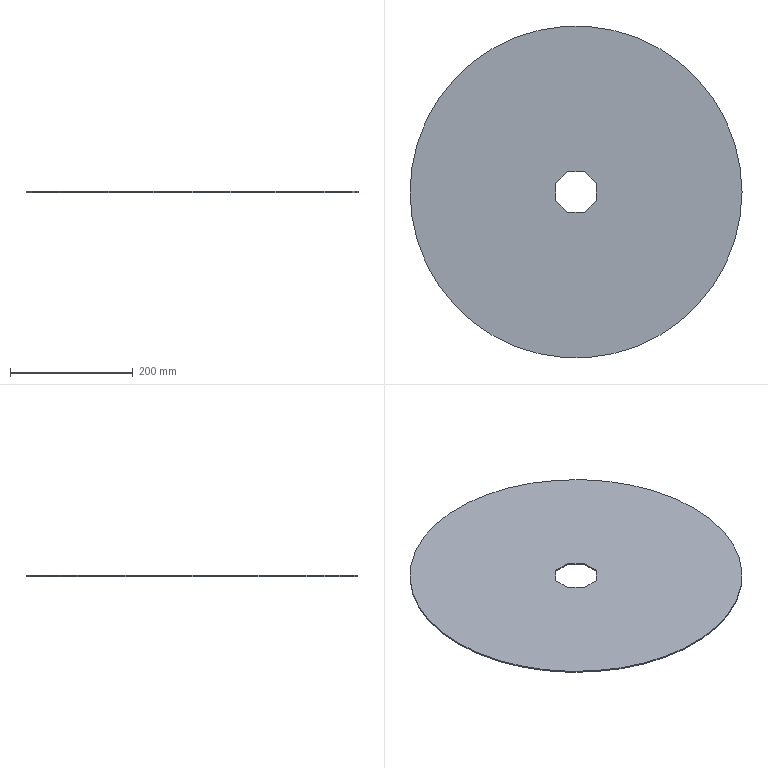Part | SolidWorks | features Extrusion 1 | 1 solid | 12 faces | box 540 x 540 x 2 mm | volume 450713 mm3 | plane 10 | cylinder 2 | commonest cylinder face diameters 540 x2
STEP:
#1=CARTESIAN_POINT('',(270.,0.,2.));
#2=VERTEX_POINT('',#1);
#3=CARTESIAN_POINT('',(-270.,0.,2.));
#4=VERTEX_POINT('',#3);
#5=CARTESIAN_POINT('',(0.,0.,2.));
#6=DIRECTION('',(0.,0.,1.));
#7=DIRECTION('',(1.,0.,0.));
#8=AXIS2_PLACEMENT_3D('',#5,#6,#7);
#9=CIRCLE('',#8,270.);
#10=EDGE_CURVE('',#2,#4,#9,.T.);
#11=ORIENTED_EDGE('',*,*,#10,.F.);
#12=CARTESIAN_POINT('',(270.,0.,0.));
#13=VERTEX_POINT('',#12);
#14=CARTESIAN_POINT('',(270.,0.,2.));
#15=DIRECTION('',(0.,0.,-1.));
#16=VECTOR('',#15,1000.);
#17=LINE('',#14,#16);
#18=EDGE_CURVE('',#2,#13,#17,.T.);
#19=ORIENTED_EDGE('',*,*,#18,.T.);
#20=CARTESIAN_POINT('',(-270.,0.,0.));
#21=VERTEX_POINT('',#20);
#22=CARTESIAN_POINT('',(0.,0.,0.));
#23=DIRECTION('',(0.,0.,1.));
#24=DIRECTION('',(1.,0.,0.));
#25=AXIS2_PLACEMENT_3D('',#22,#23,#24);
#26=CIRCLE('',#25,270.);
#27=EDGE_CURVE('',#13,#21,#26,.T.);
#28=ORIENTED_EDGE('',*,*,#27,.T.);
#29=CARTESIAN_POINT('',(-270.,0.,2.));
#30=DIRECTION('',(0.,0.,-1.));
#31=VECTOR('',#30,1000.);
#32=LINE('',#29,#31);
#33=EDGE_CURVE('',#4,#21,#32,.T.);
#34=ORIENTED_EDGE('',*,*,#33,.F.);
#35=EDGE_LOOP('',(#11,#19,#28,#34));
#36=FACE_OUTER_BOUND('',#35,.T.);
#37=CARTESIAN_POINT('',(0.,0.,2.));
#38=DIRECTION('',(0.,0.,-1.));
#39=DIRECTION('',(-1.,0.,0.));
#40=AXIS2_PLACEMENT_3D('',#37,#38,#39);
#41=CYLINDRICAL_SURFACE('',#40,270.);
#42=ADVANCED_FACE('',(#36),#41,.T.);
#43=CARTESIAN_POINT('',(0.,0.,2.));
#44=DIRECTION('',(0.,0.,1.));
#45=DIRECTION('',(1.,0.,0.));
#46=AXIS2_PLACEMENT_3D('',#43,#44,#45);
#47=CIRCLE('',#46,270.);
#48=EDGE_CURVE('',#4,#2,#47,.T.);
#49=ORIENTED_EDGE('',*,*,#48,.T.);
#50=ORIENTED_EDGE('',*,*,#10,.T.);
#51=EDGE_LOOP('',(#49,#50));
#52=FACE_OUTER_BOUND('',#51,.T.);
#53=CARTESIAN_POINT('',(-13.777,33.26,2.));
#54=VERTEX_POINT('',#53);
#55=CARTESIAN_POINT('',(-33.26,13.777,2.));
#56=VERTEX_POINT('',#55);
#57=CARTESIAN_POINT('',(-13.777,33.26,2.));
#58=DIRECTION('',(-0.7071,-0.7071,0.));
#59=VECTOR('',#58,1000.);
#60=LINE('',#57,#59);
#61=EDGE_CURVE('',#54,#56,#60,.T.);
#62=ORIENTED_EDGE('',*,*,#61,.F.);
#63=CARTESIAN_POINT('',(13.777,33.26,2.));
#64=VERTEX_POINT('',#63);
#65=CARTESIAN_POINT('',(13.777,33.26,2.));
#66=DIRECTION('',(-1.,0.,0.));
#67=VECTOR('',#66,1000.);
#68=LINE('',#65,#67);
#69=EDGE_CURVE('',#64,#54,#68,.T.);
#70=ORIENTED_EDGE('',*,*,#69,.F.);
#71=CARTESIAN_POINT('',(33.26,13.777,2.));
#72=VERTEX_POINT('',#71);
#73=CARTESIAN_POINT('',(33.26,13.777,2.));
#74=DIRECTION('',(-0.7071,0.7071,0.));
#75=VECTOR('',#74,1000.);
#76=LINE('',#73,#75);
#77=EDGE_CURVE('',#72,#64,#76,.T.);
#78=ORIENTED_EDGE('',*,*,#77,.F.);
#79=CARTESIAN_POINT('',(33.26,-13.777,2.));
#80=VERTEX_POINT('',#79);
#81=CARTESIAN_POINT('',(33.26,-13.777,2.));
#82=DIRECTION('',(0.,1.,0.));
#83=VECTOR('',#82,1000.);
#84=LINE('',#81,#83);
#85=EDGE_CURVE('',#80,#72,#84,.T.);
#86=ORIENTED_EDGE('',*,*,#85,.F.);
#87=CARTESIAN_POINT('',(13.777,-33.26,2.));
#88=VERTEX_POINT('',#87);
#89=CARTESIAN_POINT('',(13.777,-33.26,2.));
#90=DIRECTION('',(0.7071,0.7071,0.));
#91=VECTOR('',#90,1000.);
#92=LINE('',#89,#91);
#93=EDGE_CURVE('',#88,#80,#92,.T.);
#94=ORIENTED_EDGE('',*,*,#93,.F.);
#95=CARTESIAN_POINT('',(-13.777,-33.26,2.));
#96=VERTEX_POINT('',#95);
#97=CARTESIAN_POINT('',(-13.777,-33.26,2.));
#98=DIRECTION('',(1.,0.,0.));
#99=VECTOR('',#98,1000.);
#100=LINE('',#97,#99);
#101=EDGE_CURVE('',#96,#88,#100,.T.);
#102=ORIENTED_EDGE('',*,*,#101,.F.);
#103=CARTESIAN_POINT('',(-33.26,-13.777,2.));
#104=VERTEX_POINT('',#103);
#105=CARTESIAN_POINT('',(-33.26,-13.777,2.));
#106=DIRECTION('',(0.7071,-0.7071,0.));
#107=VECTOR('',#106,1000.);
#108=LINE('',#105,#107);
#109=EDGE_CURVE('',#104,#96,#108,.T.);
#110=ORIENTED_EDGE('',*,*,#109,.F.);
#111=CARTESIAN_POINT('',(-33.26,13.777,2.));
#112=DIRECTION('',(0.,-1.,0.));
#113=VECTOR('',#112,1000.);
#114=LINE('',#111,#113);
#115=EDGE_CURVE('',#56,#104,#114,.T.);
#116=ORIENTED_EDGE('',*,*,#115,.F.);
#117=EDGE_LOOP('',(#62,#70,#78,#86,#94,#102,#110,#116));
#118=FACE_BOUND('',#117,.T.);
#119=CARTESIAN_POINT('',(0.,0.,2.));
#120=DIRECTION('',(0.,0.,1.));
#121=DIRECTION('',(1.,0.,0.));
#122=AXIS2_PLACEMENT_3D('',#119,#120,#121);
#123=PLANE('',#122);
#124=ADVANCED_FACE('',(#52,#118),#123,.T.);
#125=CARTESIAN_POINT('',(0.,0.,0.));
#126=DIRECTION('',(0.,0.,1.));
#127=DIRECTION('',(1.,0.,0.));
#128=AXIS2_PLACEMENT_3D('',#125,#126,#127);
#129=CIRCLE('',#128,270.);
#130=EDGE_CURVE('',#21,#13,#129,.T.);
#131=ORIENTED_EDGE('',*,*,#130,.F.);
#132=ORIENTED_EDGE('',*,*,#27,.F.);
#133=EDGE_LOOP('',(#131,#132));
#134=FACE_OUTER_BOUND('',#133,.T.);
#135=CARTESIAN_POINT('',(13.777,33.26,0.));
#136=VERTEX_POINT('',#135);
#137=CARTESIAN_POINT('',(-13.777,33.26,0.));
#138=VERTEX_POINT('',#137);
#139=CARTESIAN_POINT('',(13.777,33.26,0.));
#140=DIRECTION('',(-1.,0.,0.));
#141=VECTOR('',#140,1000.);
#142=LINE('',#139,#141);
#143=EDGE_CURVE('',#136,#138,#142,.T.);
#144=ORIENTED_EDGE('',*,*,#143,.T.);
#145=CARTESIAN_POINT('',(-33.26,13.777,0.));
#146=VERTEX_POINT('',#145);
#147=CARTESIAN_POINT('',(-13.777,33.26,0.));
#148=DIRECTION('',(-0.7071,-0.7071,0.));
#149=VECTOR('',#148,1000.);
#150=LINE('',#147,#149);
#151=EDGE_CURVE('',#138,#146,#150,.T.);
#152=ORIENTED_EDGE('',*,*,#151,.T.);
#153=CARTESIAN_POINT('',(-33.26,-13.777,0.));
#154=VERTEX_POINT('',#153);
#155=CARTESIAN_POINT('',(-33.26,13.777,0.));
#156=DIRECTION('',(0.,-1.,0.));
#157=VECTOR('',#156,1000.);
#158=LINE('',#155,#157);
#159=EDGE_CURVE('',#146,#154,#158,.T.);
#160=ORIENTED_EDGE('',*,*,#159,.T.);
#161=CARTESIAN_POINT('',(-13.777,-33.26,0.));
#162=VERTEX_POINT('',#161);
#163=CARTESIAN_POINT('',(-33.26,-13.777,0.));
#164=DIRECTION('',(0.7071,-0.7071,0.));
#165=VECTOR('',#164,1000.);
#166=LINE('',#163,#165);
#167=EDGE_CURVE('',#154,#162,#166,.T.);
#168=ORIENTED_EDGE('',*,*,#167,.T.);
#169=CARTESIAN_POINT('',(13.777,-33.26,0.));
#170=VERTEX_POINT('',#169);
#171=CARTESIAN_POINT('',(-13.777,-33.26,0.));
#172=DIRECTION('',(1.,0.,0.));
#173=VECTOR('',#172,1000.);
#174=LINE('',#171,#173);
#175=EDGE_CURVE('',#162,#170,#174,.T.);
#176=ORIENTED_EDGE('',*,*,#175,.T.);
#177=CARTESIAN_POINT('',(33.26,-13.777,0.));
#178=VERTEX_POINT('',#177);
#179=CARTESIAN_POINT('',(13.777,-33.26,0.));
#180=DIRECTION('',(0.7071,0.7071,0.));
#181=VECTOR('',#180,1000.);
#182=LINE('',#179,#181);
#183=EDGE_CURVE('',#170,#178,#182,.T.);
#184=ORIENTED_EDGE('',*,*,#183,.T.);
#185=CARTESIAN_POINT('',(33.26,13.777,0.));
#186=VERTEX_POINT('',#185);
#187=CARTESIAN_POINT('',(33.26,-13.777,0.));
#188=DIRECTION('',(0.,1.,0.));
#189=VECTOR('',#188,1000.);
#190=LINE('',#187,#189);
#191=EDGE_CURVE('',#178,#186,#190,.T.);
#192=ORIENTED_EDGE('',*,*,#191,.T.);
#193=CARTESIAN_POINT('',(33.26,13.777,0.));
#194=DIRECTION('',(-0.7071,0.7071,0.));
#195=VECTOR('',#194,1000.);
#196=LINE('',#193,#195);
#197=EDGE_CURVE('',#186,#136,#196,.T.);
#198=ORIENTED_EDGE('',*,*,#197,.T.);
#199=EDGE_LOOP('',(#144,#152,#160,#168,#176,#184,#192,#198));
#200=FACE_BOUND('',#199,.T.);
#201=CARTESIAN_POINT('',(0.,0.,0.));
#202=DIRECTION('',(0.,0.,1.));
#203=DIRECTION('',(1.,0.,0.));
#204=AXIS2_PLACEMENT_3D('',#201,#202,#203);
#205=PLANE('',#204);
#206=ADVANCED_FACE('',(#134,#200),#205,.F.);
#207=ORIENTED_EDGE('',*,*,#18,.F.);
#208=ORIENTED_EDGE('',*,*,#48,.F.);
#209=ORIENTED_EDGE('',*,*,#33,.T.);
#210=ORIENTED_EDGE('',*,*,#130,.T.);
#211=EDGE_LOOP('',(#207,#208,#209,#210));
#212=FACE_OUTER_BOUND('',#211,.T.);
#213=CARTESIAN_POINT('',(0.,0.,2.));
#214=DIRECTION('',(0.,0.,-1.));
#215=DIRECTION('',(-1.,0.,0.));
#216=AXIS2_PLACEMENT_3D('',#213,#214,#215);
#217=CYLINDRICAL_SURFACE('',#216,270.);
#218=ADVANCED_FACE('',(#212),#217,.T.);
#219=ORIENTED_EDGE('',*,*,#143,.F.);
#220=CARTESIAN_POINT('',(13.777,33.26,2.));
#221=DIRECTION('',(0.,0.,-1.));
#222=VECTOR('',#221,1000.);
#223=LINE('',#220,#222);
#224=EDGE_CURVE('',#64,#136,#223,.T.);
#225=ORIENTED_EDGE('',*,*,#224,.F.);
#226=ORIENTED_EDGE('',*,*,#69,.T.);
#227=CARTESIAN_POINT('',(-13.777,33.26,2.));
#228=DIRECTION('',(0.,0.,-1.));
#229=VECTOR('',#228,1000.);
#230=LINE('',#227,#229);
#231=EDGE_CURVE('',#54,#138,#230,.T.);
#232=ORIENTED_EDGE('',*,*,#231,.T.);
#233=EDGE_LOOP('',(#219,#225,#226,#232));
#234=FACE_OUTER_BOUND('',#233,.T.);
#235=CARTESIAN_POINT('',(13.777,33.26,2.));
#236=DIRECTION('',(0.,-1.,0.));
#237=DIRECTION('',(1.,0.,0.));
#238=AXIS2_PLACEMENT_3D('',#235,#236,#237);
#239=PLANE('',#238);
#240=ADVANCED_FACE('',(#234),#239,.T.);
#241=ORIENTED_EDGE('',*,*,#151,.F.);
#242=ORIENTED_EDGE('',*,*,#231,.F.);
#243=ORIENTED_EDGE('',*,*,#61,.T.);
#244=CARTESIAN_POINT('',(-33.26,13.777,2.));
#245=DIRECTION('',(0.,0.,-1.));
#246=VECTOR('',#245,1000.);
#247=LINE('',#244,#246);
#248=EDGE_CURVE('',#56,#146,#247,.T.);
#249=ORIENTED_EDGE('',*,*,#248,.T.);
#250=EDGE_LOOP('',(#241,#242,#243,#249));
#251=FACE_OUTER_BOUND('',#250,.T.);
#252=CARTESIAN_POINT('',(-13.777,33.26,2.));
#253=DIRECTION('',(0.7071,-0.7071,0.));
#254=DIRECTION('',(0.7071,0.7071,0.));
#255=AXIS2_PLACEMENT_3D('',#252,#253,#254);
#256=PLANE('',#255);
#257=ADVANCED_FACE('',(#251),#256,.T.);
#258=ORIENTED_EDGE('',*,*,#159,.F.);
#259=ORIENTED_EDGE('',*,*,#248,.F.);
#260=ORIENTED_EDGE('',*,*,#115,.T.);
#261=CARTESIAN_POINT('',(-33.26,-13.777,2.));
#262=DIRECTION('',(0.,0.,-1.));
#263=VECTOR('',#262,1000.);
#264=LINE('',#261,#263);
#265=EDGE_CURVE('',#104,#154,#264,.T.);
#266=ORIENTED_EDGE('',*,*,#265,.T.);
#267=EDGE_LOOP('',(#258,#259,#260,#266));
#268=FACE_OUTER_BOUND('',#267,.T.);
#269=CARTESIAN_POINT('',(-33.26,13.777,2.));
#270=DIRECTION('',(1.,0.,0.));
#271=DIRECTION('',(0.,1.,0.));
#272=AXIS2_PLACEMENT_3D('',#269,#270,#271);
#273=PLANE('',#272);
#274=ADVANCED_FACE('',(#268),#273,.T.);
#275=ORIENTED_EDGE('',*,*,#167,.F.);
#276=ORIENTED_EDGE('',*,*,#265,.F.);
#277=ORIENTED_EDGE('',*,*,#109,.T.);
#278=CARTESIAN_POINT('',(-13.777,-33.26,2.));
#279=DIRECTION('',(0.,0.,-1.));
#280=VECTOR('',#279,1000.);
#281=LINE('',#278,#280);
#282=EDGE_CURVE('',#96,#162,#281,.T.);
#283=ORIENTED_EDGE('',*,*,#282,.T.);
#284=EDGE_LOOP('',(#275,#276,#277,#283));
#285=FACE_OUTER_BOUND('',#284,.T.);
#286=CARTESIAN_POINT('',(-33.26,-13.777,2.));
#287=DIRECTION('',(0.7071,0.7071,0.));
#288=DIRECTION('',(-0.7071,0.7071,0.));
#289=AXIS2_PLACEMENT_3D('',#286,#287,#288);
#290=PLANE('',#289);
#291=ADVANCED_FACE('',(#285),#290,.T.);
#292=ORIENTED_EDGE('',*,*,#175,.F.);
#293=ORIENTED_EDGE('',*,*,#282,.F.);
#294=ORIENTED_EDGE('',*,*,#101,.T.);
#295=CARTESIAN_POINT('',(13.777,-33.26,2.));
#296=DIRECTION('',(0.,0.,-1.));
#297=VECTOR('',#296,1000.);
#298=LINE('',#295,#297);
#299=EDGE_CURVE('',#88,#170,#298,.T.);
#300=ORIENTED_EDGE('',*,*,#299,.T.);
#301=EDGE_LOOP('',(#292,#293,#294,#300));
#302=FACE_OUTER_BOUND('',#301,.T.);
#303=CARTESIAN_POINT('',(-13.777,-33.26,2.));
#304=DIRECTION('',(0.,1.,0.));
#305=DIRECTION('',(-1.,0.,0.));
#306=AXIS2_PLACEMENT_3D('',#303,#304,#305);
#307=PLANE('',#306);
#308=ADVANCED_FACE('',(#302),#307,.T.);
#309=ORIENTED_EDGE('',*,*,#183,.F.);
#310=ORIENTED_EDGE('',*,*,#299,.F.);
#311=ORIENTED_EDGE('',*,*,#93,.T.);
#312=CARTESIAN_POINT('',(33.26,-13.777,2.));
#313=DIRECTION('',(0.,0.,-1.));
#314=VECTOR('',#313,1000.);
#315=LINE('',#312,#314);
#316=EDGE_CURVE('',#80,#178,#315,.T.);
#317=ORIENTED_EDGE('',*,*,#316,.T.);
#318=EDGE_LOOP('',(#309,#310,#311,#317));
#319=FACE_OUTER_BOUND('',#318,.T.);
#320=CARTESIAN_POINT('',(13.777,-33.26,2.));
#321=DIRECTION('',(-0.7071,0.7071,0.));
#322=DIRECTION('',(-0.7071,-0.7071,0.));
#323=AXIS2_PLACEMENT_3D('',#320,#321,#322);
#324=PLANE('',#323);
#325=ADVANCED_FACE('',(#319),#324,.T.);
#326=ORIENTED_EDGE('',*,*,#191,.F.);
#327=ORIENTED_EDGE('',*,*,#316,.F.);
#328=ORIENTED_EDGE('',*,*,#85,.T.);
#329=CARTESIAN_POINT('',(33.26,13.777,2.));
#330=DIRECTION('',(0.,0.,-1.));
#331=VECTOR('',#330,1000.);
#332=LINE('',#329,#331);
#333=EDGE_CURVE('',#72,#186,#332,.T.);
#334=ORIENTED_EDGE('',*,*,#333,.T.);
#335=EDGE_LOOP('',(#326,#327,#328,#334));
#336=FACE_OUTER_BOUND('',#335,.T.);
#337=CARTESIAN_POINT('',(33.26,-13.777,2.));
#338=DIRECTION('',(-1.,0.,0.));
#339=DIRECTION('',(0.,0.,1.));
#340=AXIS2_PLACEMENT_3D('',#337,#338,#339);
#341=PLANE('',#340);
#342=ADVANCED_FACE('',(#336),#341,.T.);
#343=ORIENTED_EDGE('',*,*,#197,.F.);
#344=ORIENTED_EDGE('',*,*,#333,.F.);
#345=ORIENTED_EDGE('',*,*,#77,.T.);
#346=ORIENTED_EDGE('',*,*,#224,.T.);
#347=EDGE_LOOP('',(#343,#344,#345,#346));
#348=FACE_OUTER_BOUND('',#347,.T.);
#349=CARTESIAN_POINT('',(33.26,13.777,2.));
#350=DIRECTION('',(-0.7071,-0.7071,0.));
#351=DIRECTION('',(0.7071,-0.7071,0.));
#352=AXIS2_PLACEMENT_3D('',#349,#350,#351);
#353=PLANE('',#352);
#354=ADVANCED_FACE('',(#348),#353,.T.);
#355=CLOSED_SHELL('',(#42,#124,#206,#218,#240,#257,#274,#291,#308,#325,#342,#354));
#356=MANIFOLD_SOLID_BREP('',#355);
#357=CARTESIAN_POINT('',(0.,0.,0.));
#358=DIRECTION('',(0.,0.,1.));
#359=DIRECTION('',(1.,0.,0.));
#360=AXIS2_PLACEMENT_3D('',#357,#358,#359);
#361=(LENGTH_UNIT()NAMED_UNIT(*)SI_UNIT(.MILLI.,.METRE.));
#362=UNCERTAINTY_MEASURE_WITH_UNIT(LENGTH_MEASURE(0.00001),#361,'','');
#363=(NAMED_UNIT(*)PLANE_ANGLE_UNIT()SI_UNIT($,.RADIAN.));
#364=(NAMED_UNIT(*)SI_UNIT($,.STERADIAN.)SOLID_ANGLE_UNIT());
#365=(GEOMETRIC_REPRESENTATION_CONTEXT(3)GLOBAL_UNCERTAINTY_ASSIGNED_CONTEXT((#362))GLOBAL_UNIT_ASSIGNED_CONTEXT((#361,#363,#364))REPRESENTATION_CONTEXT('',''));
#366=ADVANCED_BREP_SHAPE_REPRESENTATION('',(#356,#360),#365);